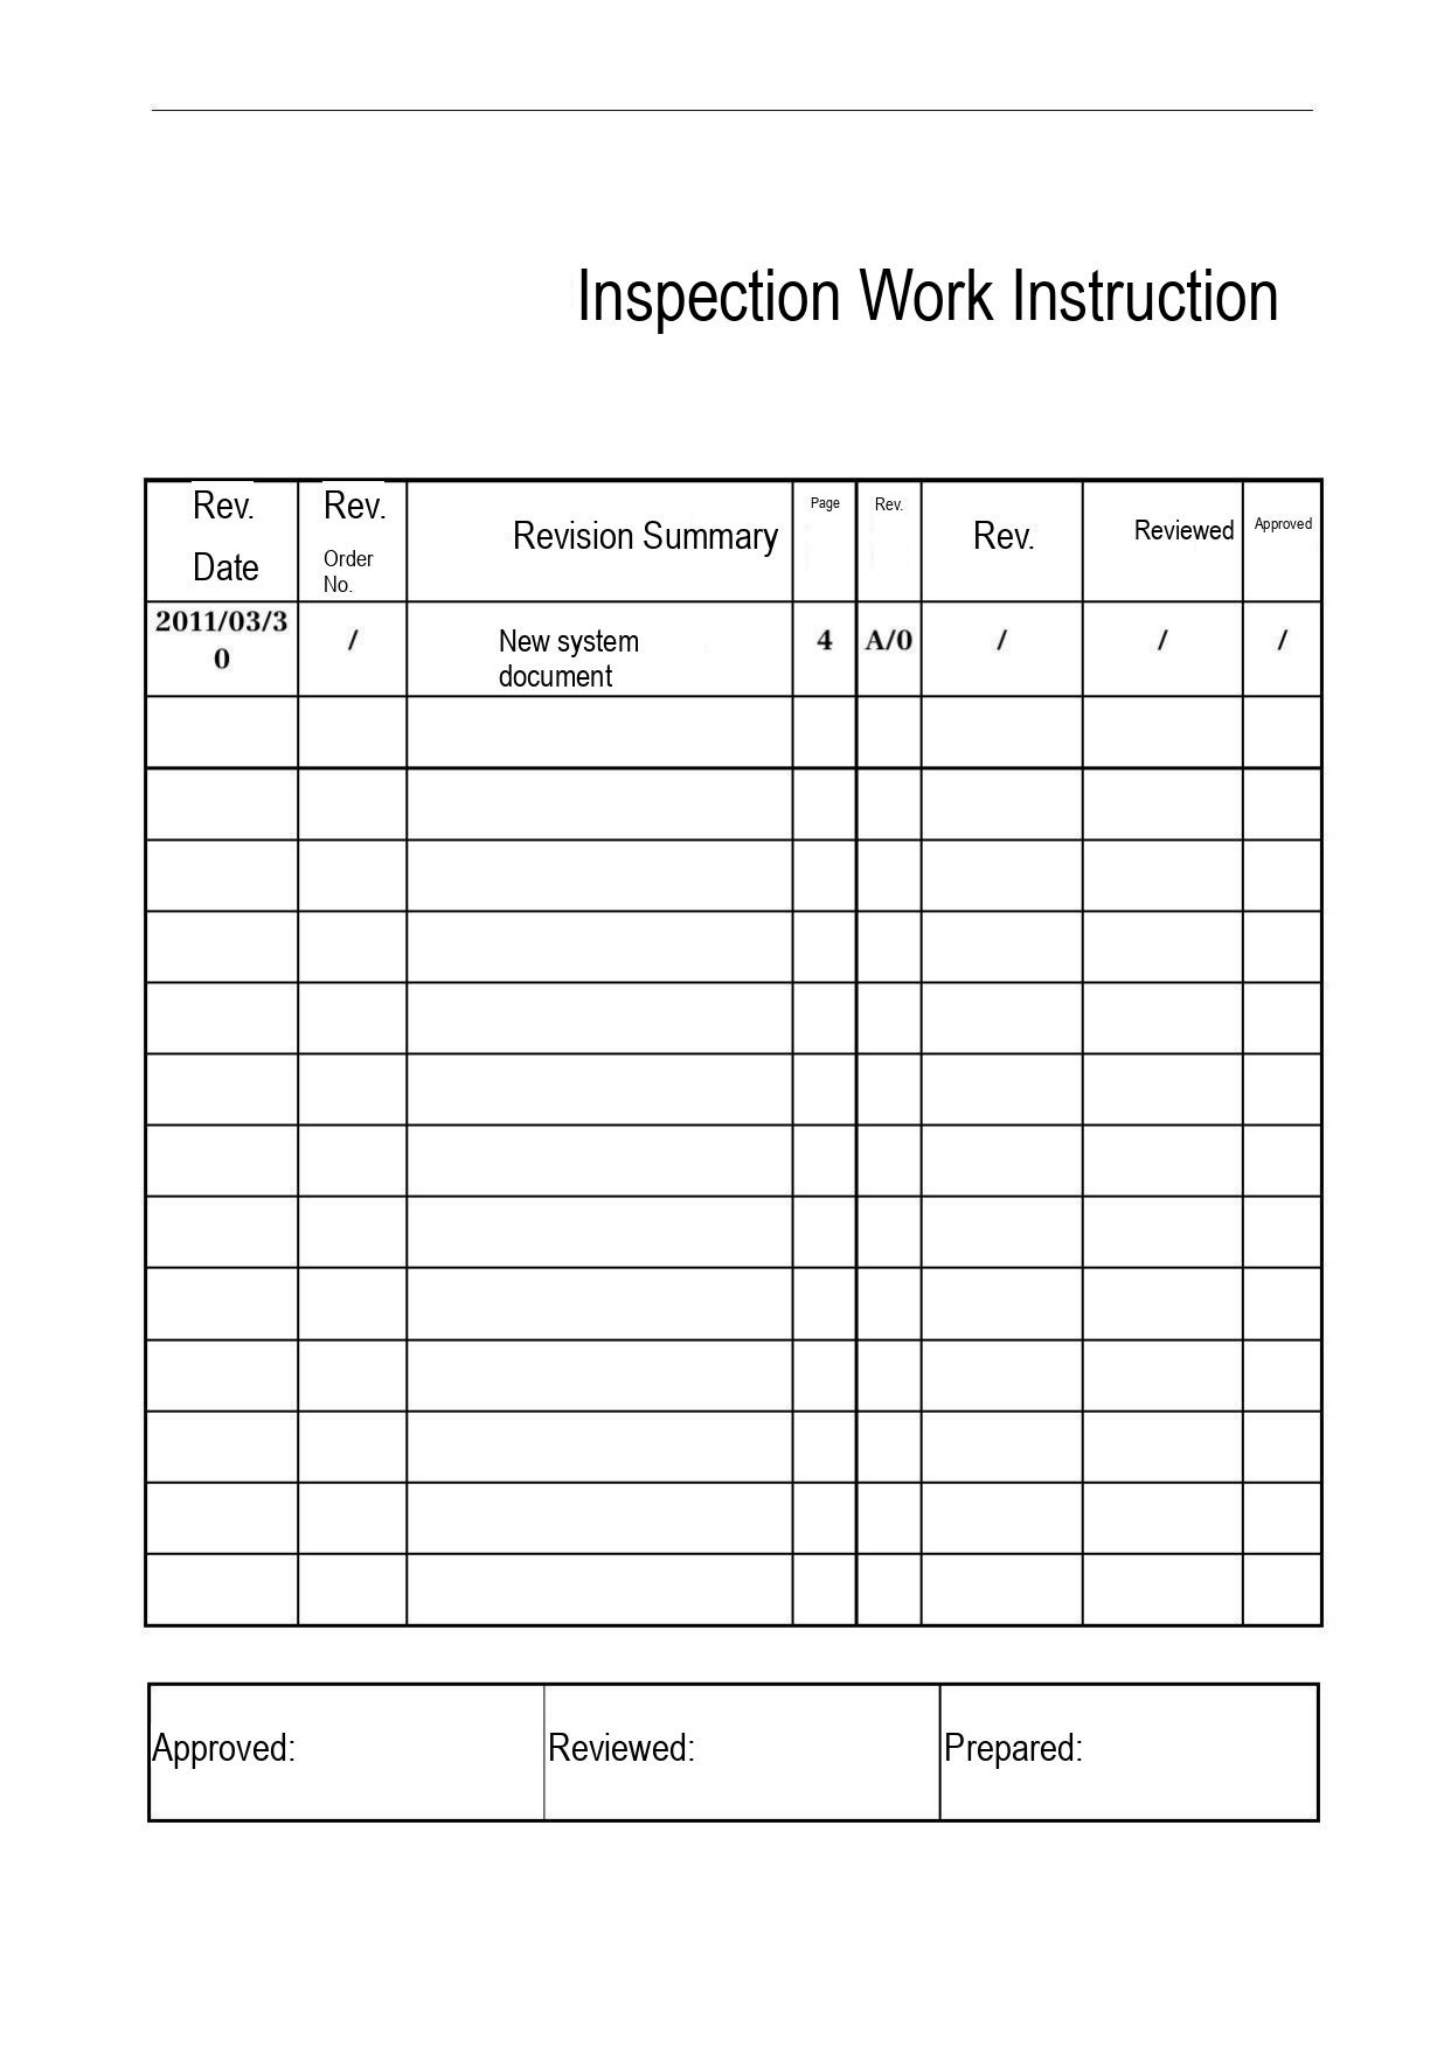Inspection Work Instruction

| Rev. Date | Rev. Order No. | Revision Summary | Page | Rev. | Rev. | Reviewed | Approved |
|---|---|---|---|---|---|---|---|
| 2011/03/30 | / | New system document | 4 | A/0 | / | / | / |
| | | | | | | | |
| | | | | | | | |
| | | | | | | | |
| | | | | | | | |
| | | | | | | | |
| | | | | | | | |
| | | | | | | | |
| | | | | | | | |
| | | | | | | | |
| | | | | | | | |
| | | | | | | | |
| | | | | | | | |
| | | | | | | | |

| Approved: | Reviewed: | Prepared: |
|---|---|---|
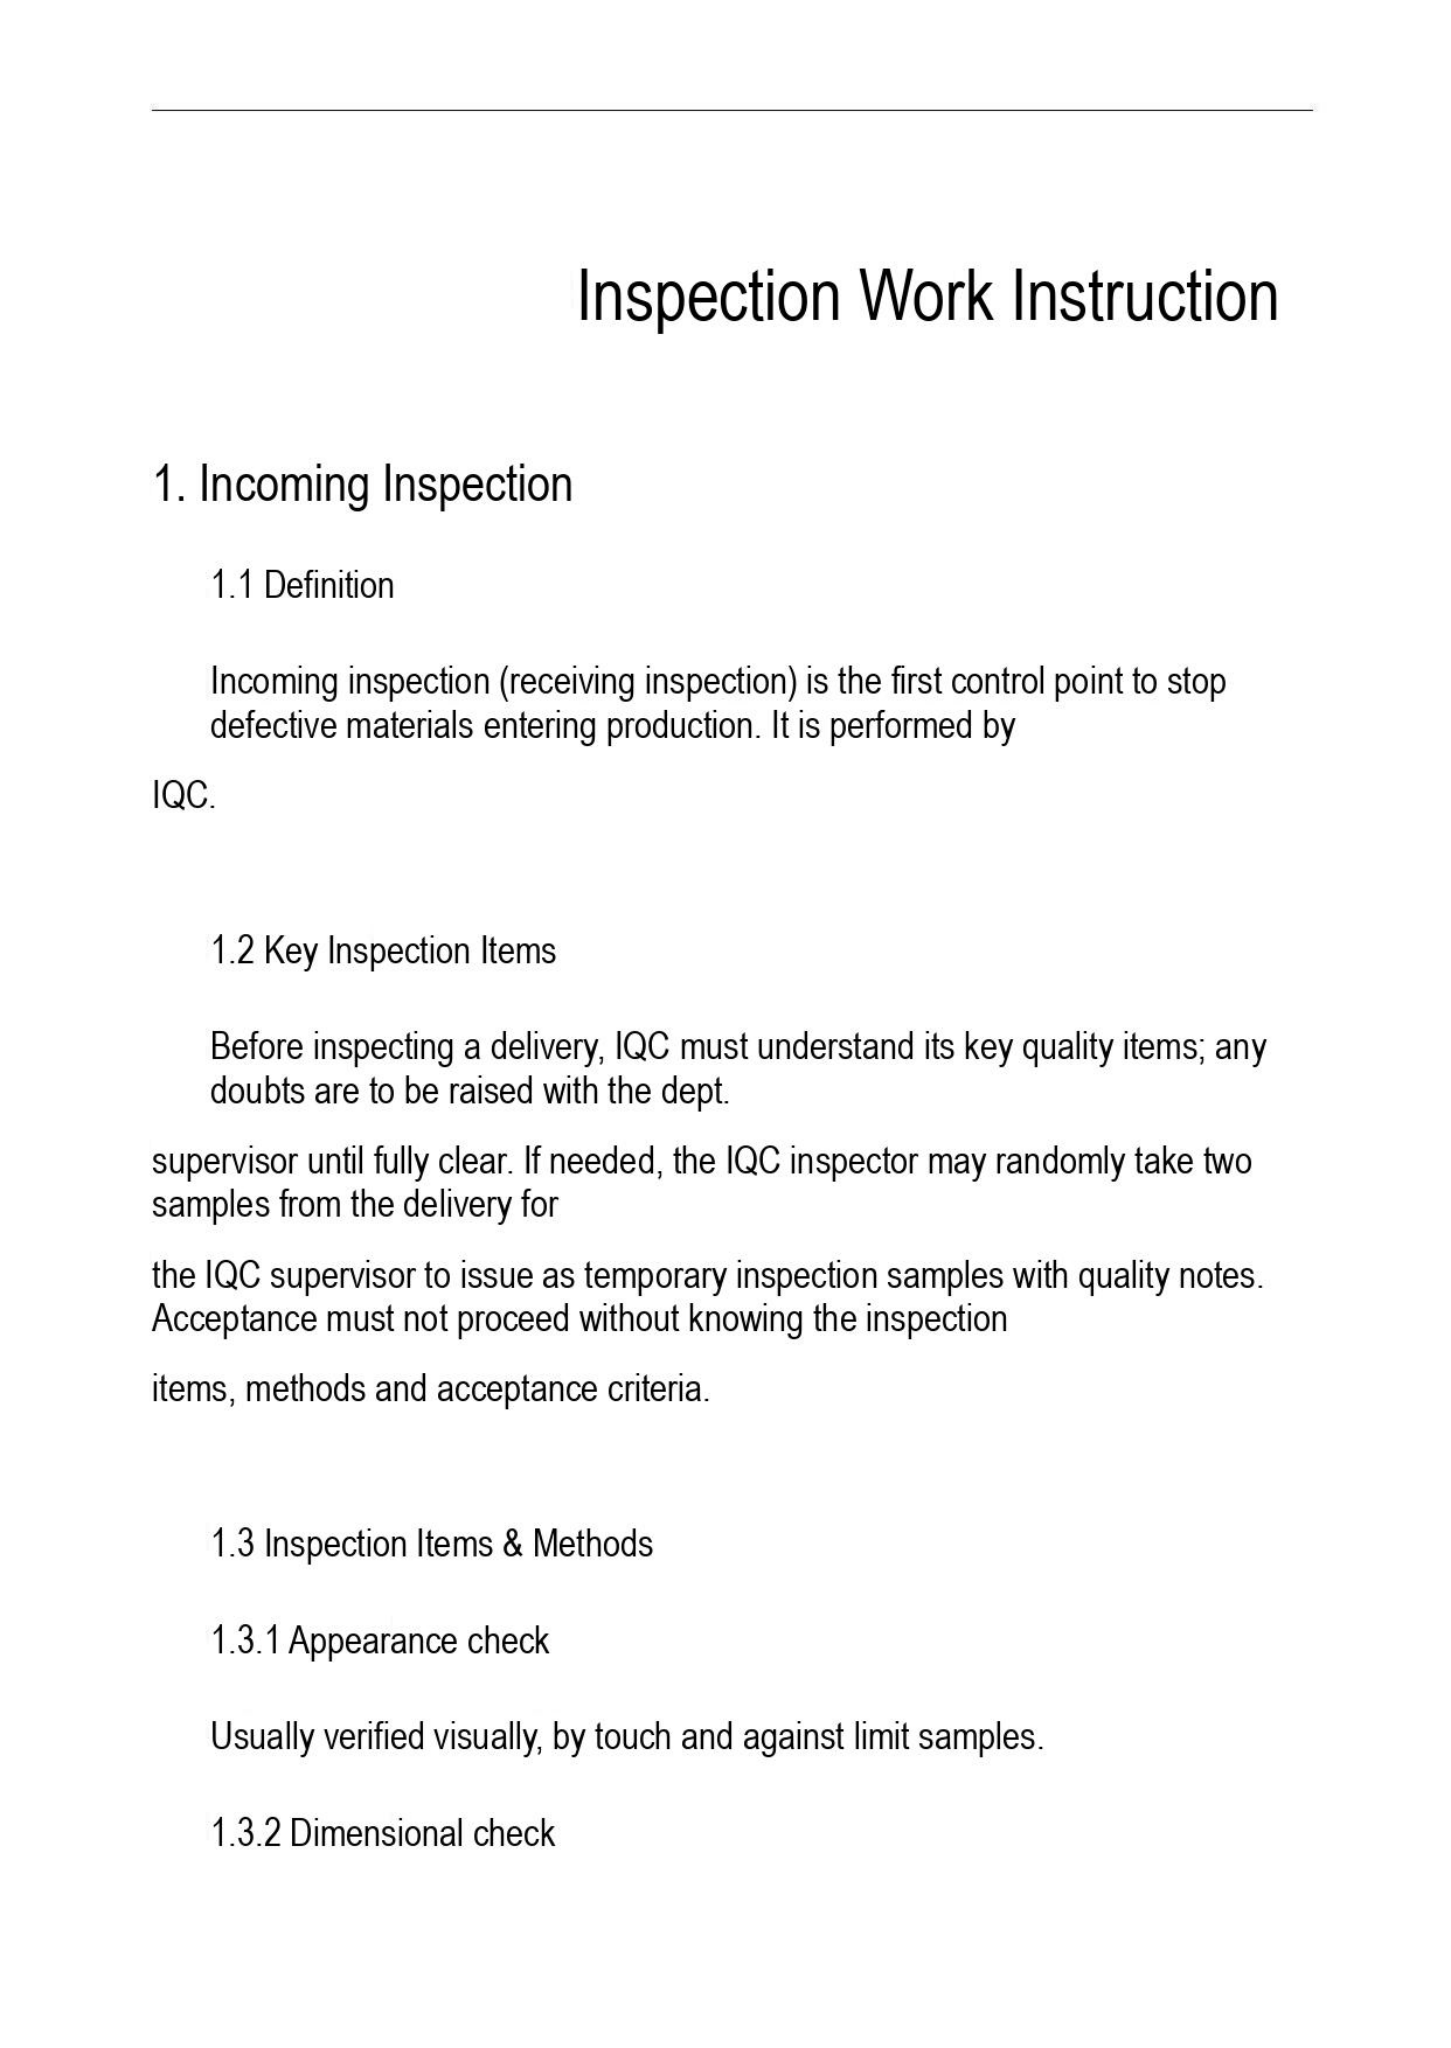Inspection Work Instruction

1. Incoming Inspection

1.1 Definition

Incoming inspection (receiving inspection) is the first control point to stop defective materials entering production. It is performed by IQC.

1.2 Key Inspection Items

Before inspecting a delivery, IQC must understand its key quality items; any doubts are to be raised with the dept. supervisor until fully clear. If needed, the IQC inspector may randomly take two samples from the delivery for the IQC supervisor to issue as temporary inspection samples with quality notes. Acceptance must not proceed without knowing the inspection items, methods and acceptance criteria.

1.3 Inspection Items & Methods

1.3.1 Appearance check

Usually verified visually, by touch and against limit samples.

1.3.2 Dimensional check
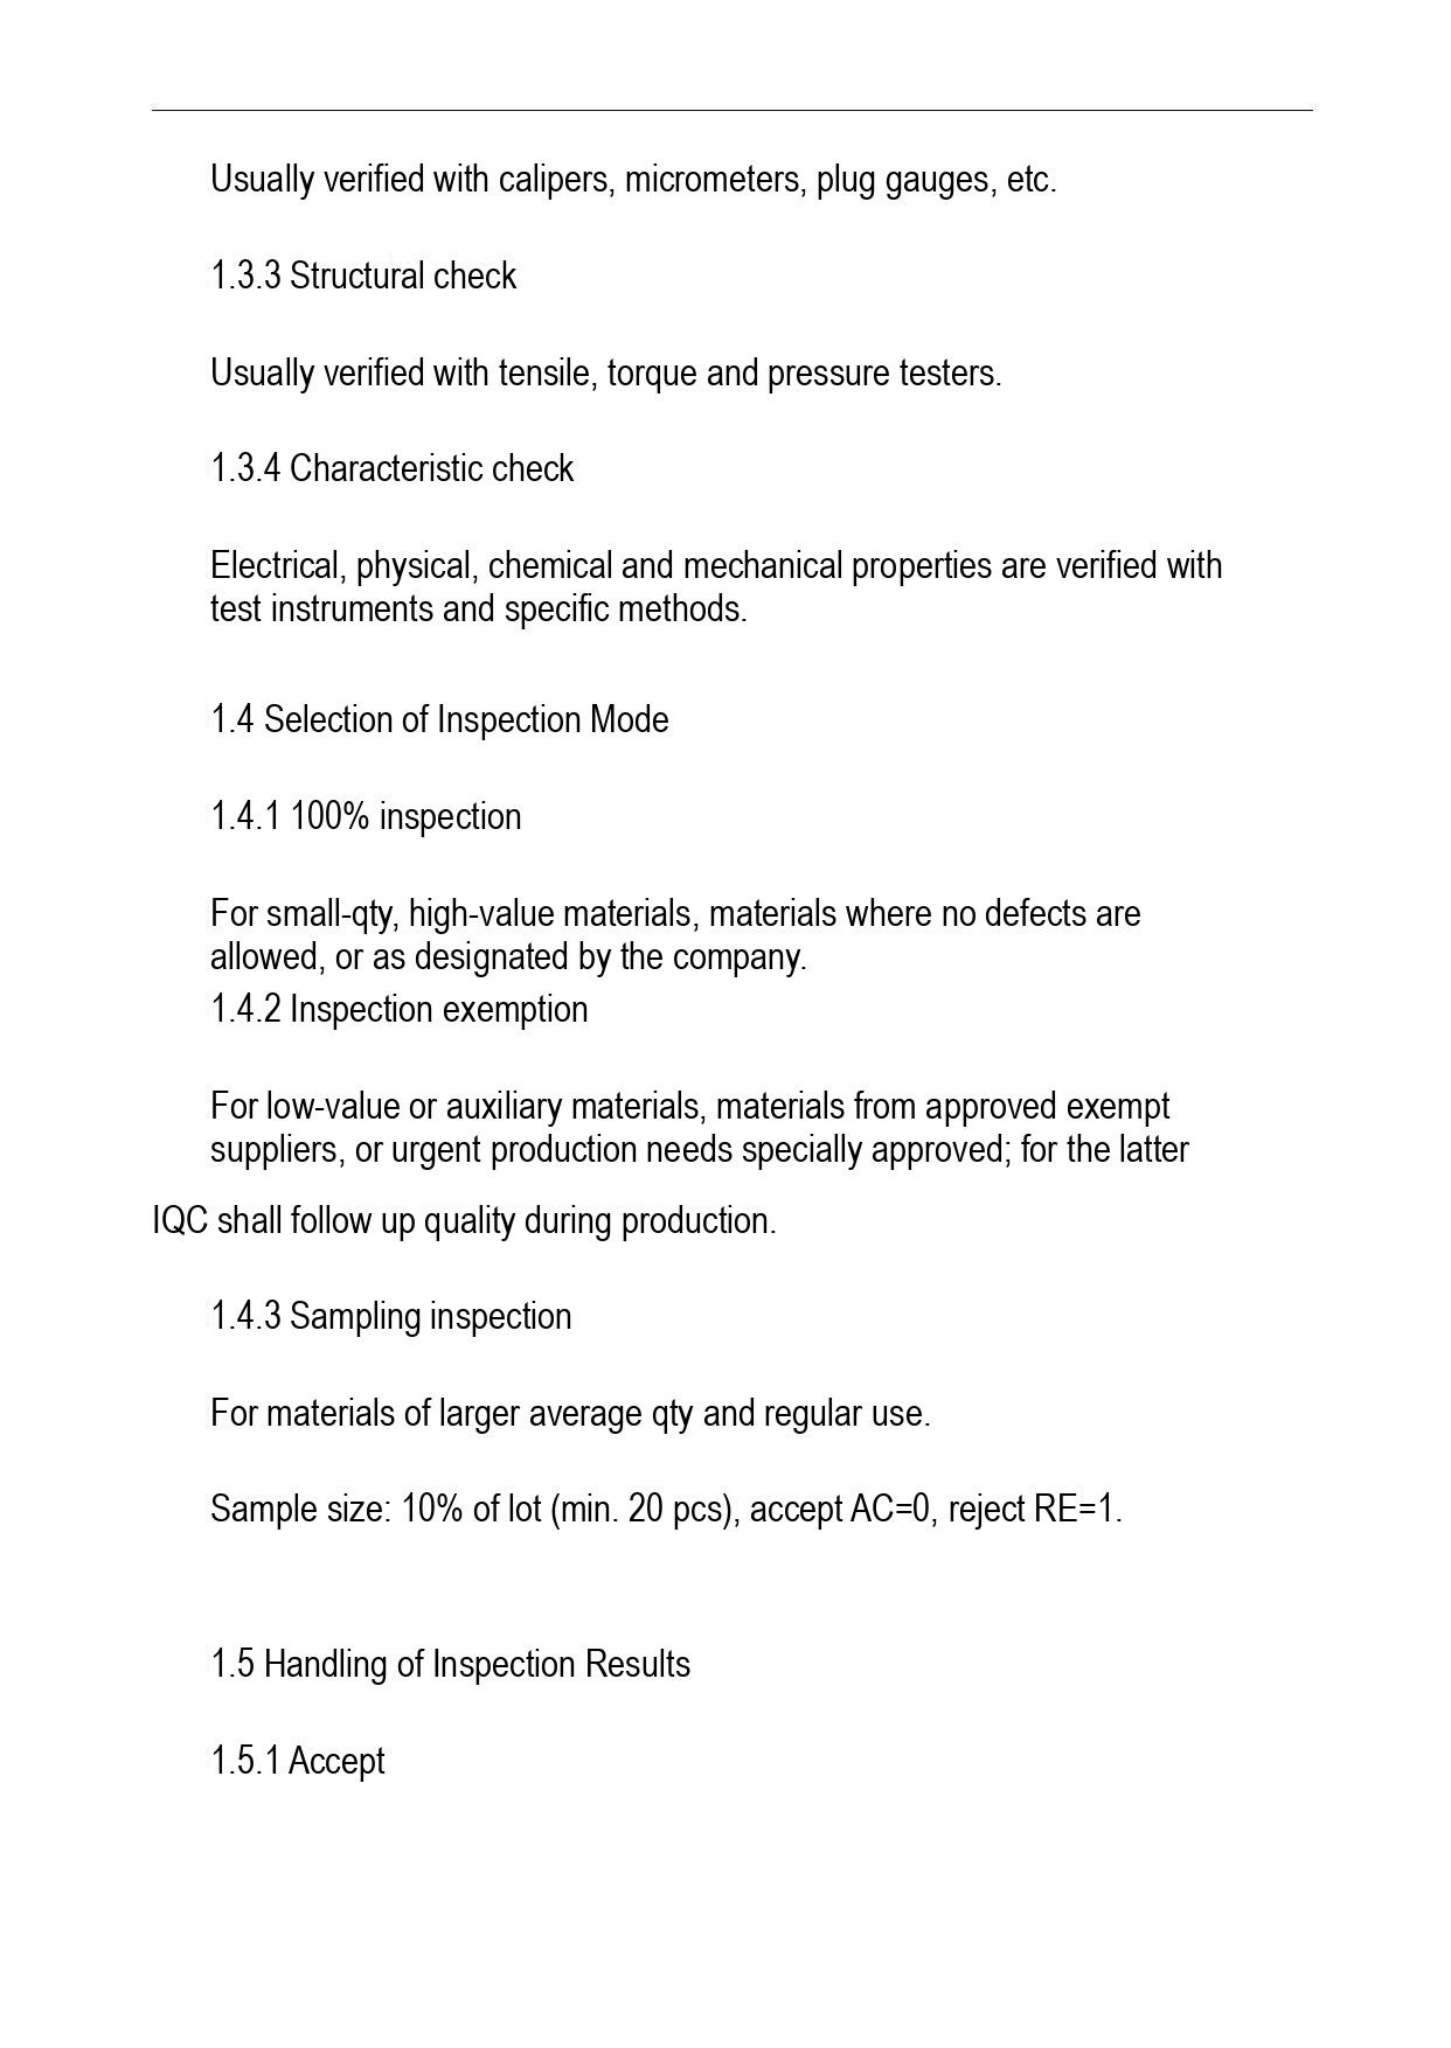Usually verified with calipers, micrometers, plug gauges, etc.

1.3.3 Structural check

Usually verified with tensile, torque and pressure testers.

1.3.4 Characteristic check

Electrical, physical, chemical and mechanical properties are verified with test instruments and specific methods.

1.4 Selection of Inspection Mode

1.4.1 100% inspection

For small-qty, high-value materials, materials where no defects are allowed, or as designated by the company.
1.4.2 Inspection exemption

For low-value or auxiliary materials, materials from approved exempt suppliers, or urgent production needs specially approved; for the latter

IQC shall follow up quality during production.

1.4.3 Sampling inspection

For materials of larger average qty and regular use.

Sample size: 10% of lot (min. 20 pcs), accept AC=0, reject RE=1.

1.5 Handling of Inspection Results

1.5.1 Accept
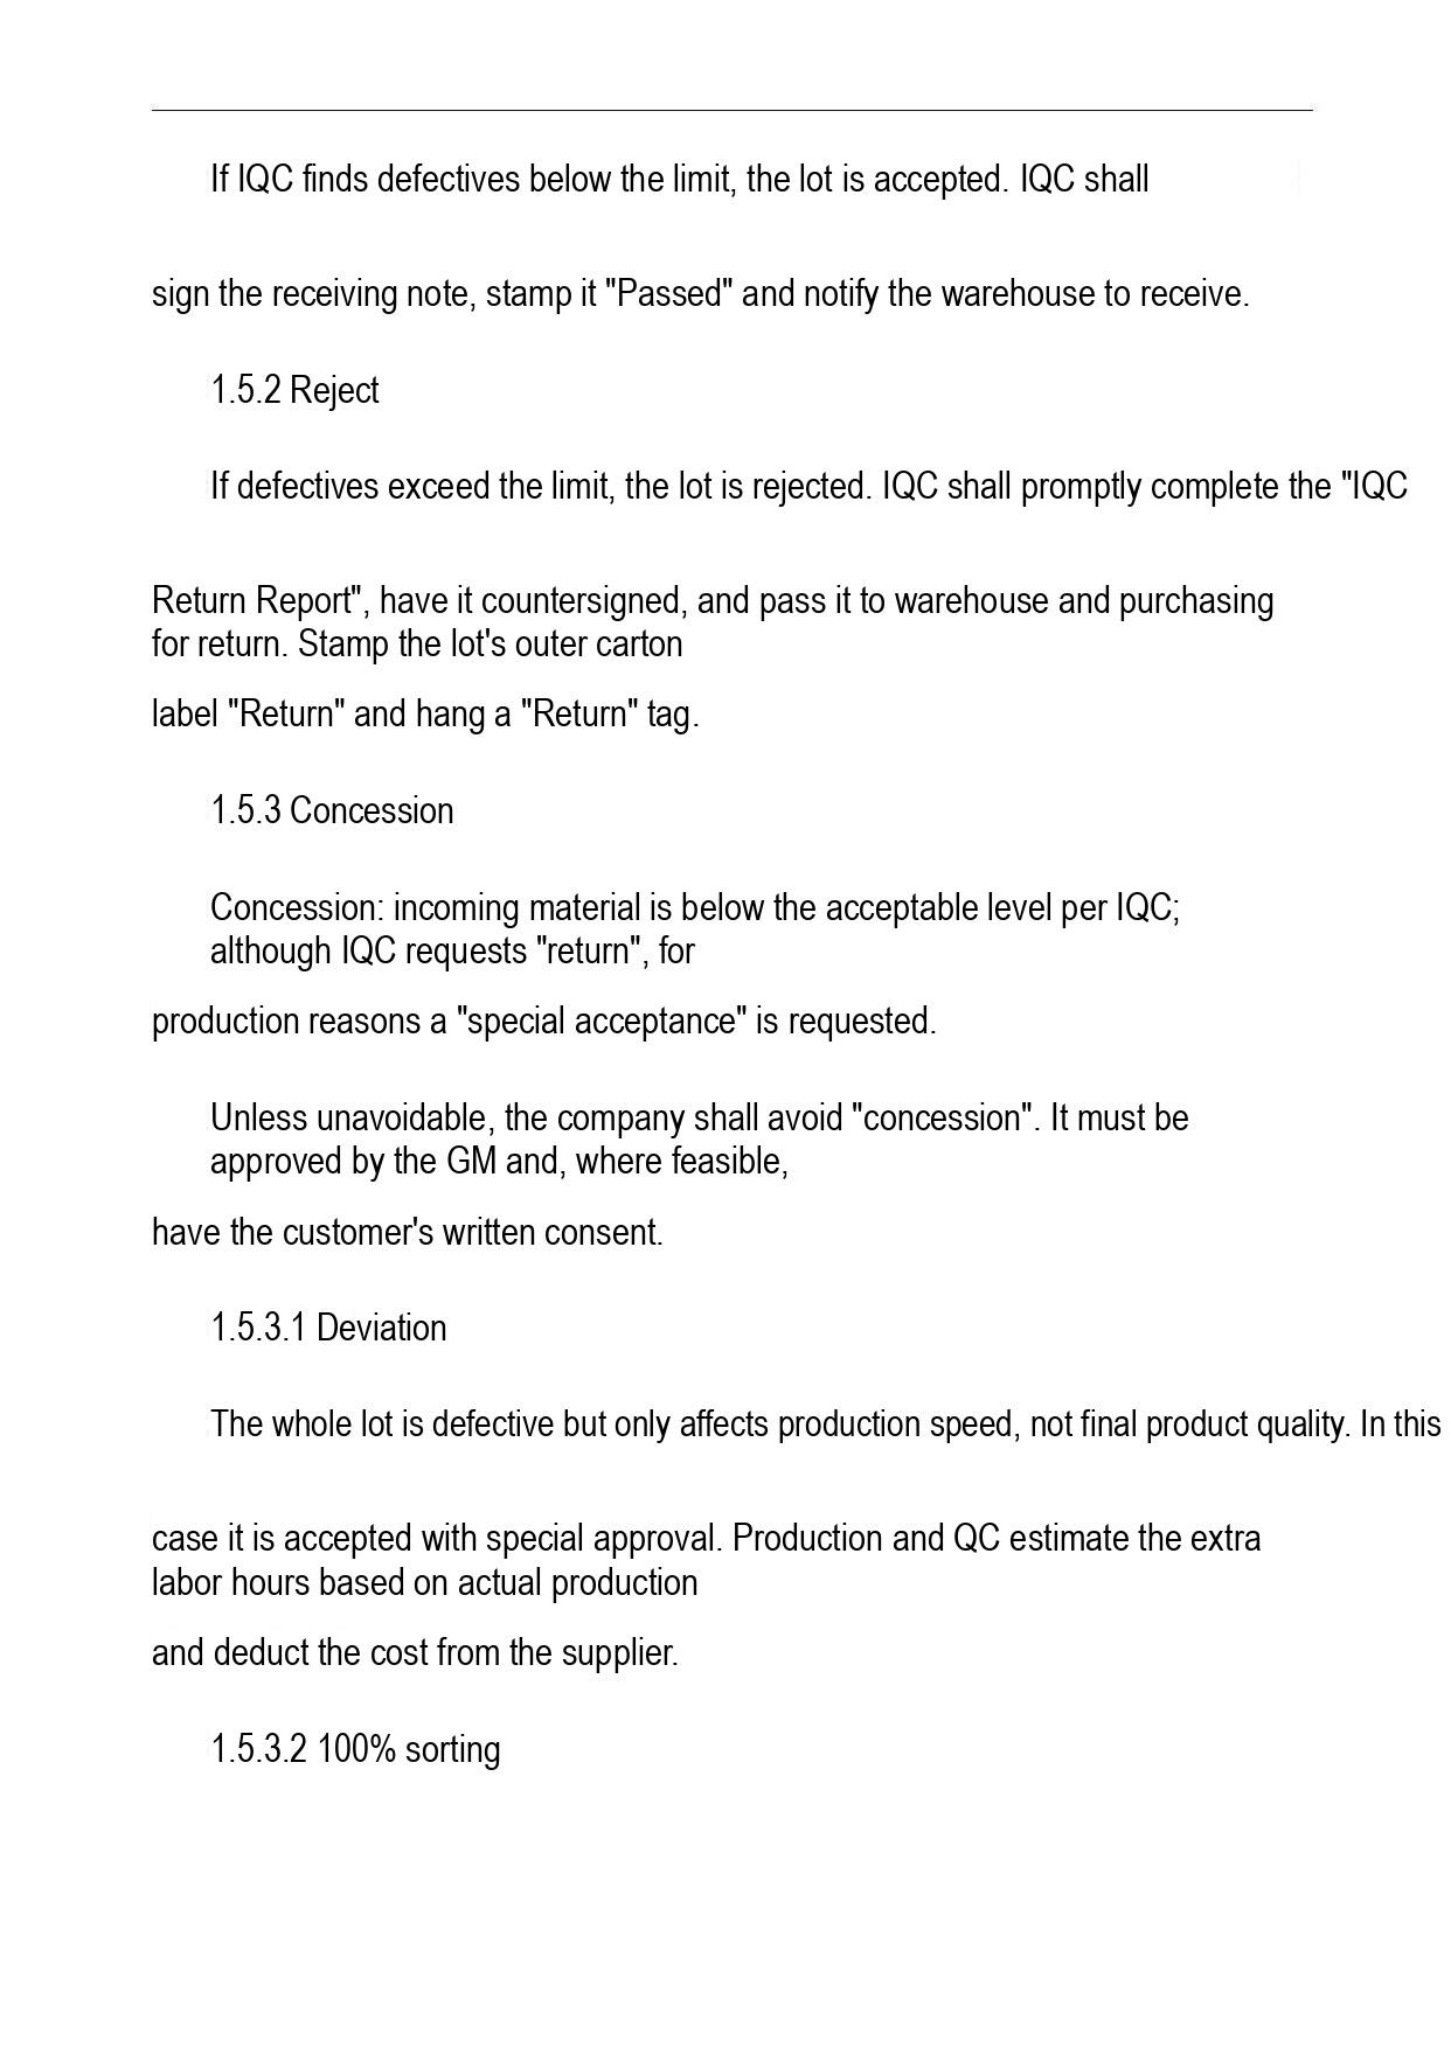If IQC finds defectives below the limit, the lot is accepted. IQC shall sign the receiving note, stamp it "Passed" and notify the warehouse to receive.

1.5.2 Reject

If defectives exceed the limit, the lot is rejected. IQC shall promptly complete the "IQC Return Report", have it countersigned, and pass it to warehouse and purchasing for return. Stamp the lot's outer carton label "Return" and hang a "Return" tag.

1.5.3 Concession

Concession: incoming material is below the acceptable level per IQC; although IQC requests "return", for production reasons a "special acceptance" is requested.

Unless unavoidable, the company shall avoid "concession". It must be approved by the GM and, where feasible, have the customer's written consent.

1.5.3.1 Deviation

The whole lot is defective but only affects production speed, not final product quality. In this case it is accepted with special approval. Production and QC estimate the extra labor hours based on actual production and deduct the cost from the supplier.

1.5.3.2 100% sorting
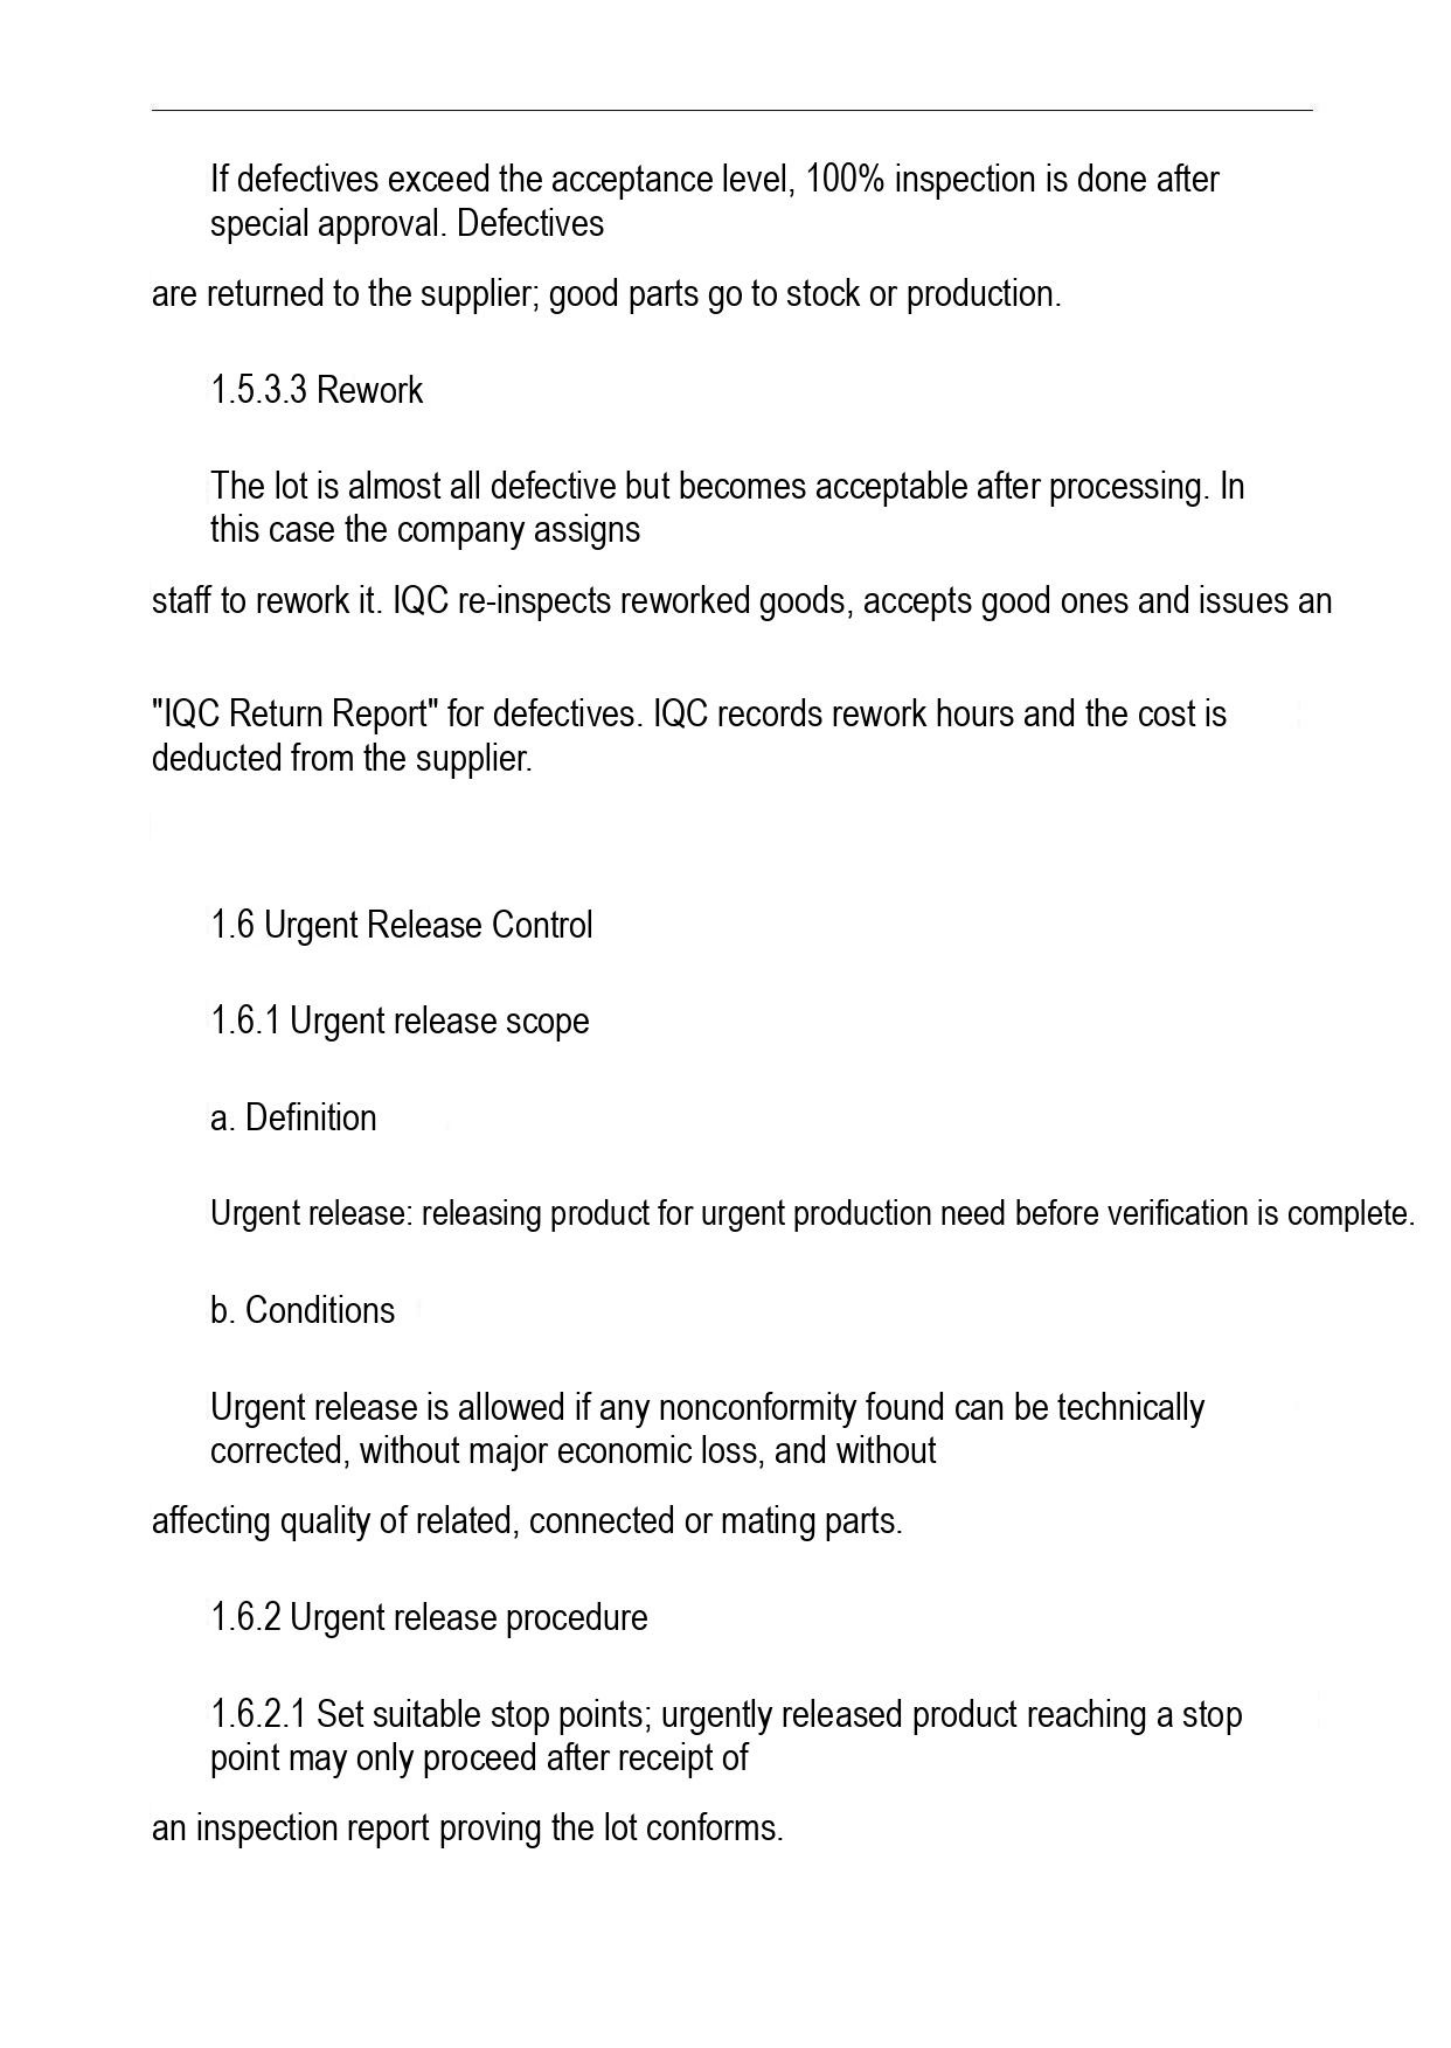If defectives exceed the acceptance level, 100% inspection is done after special approval. Defectives are returned to the supplier; good parts go to stock or production.

1.5.3.3 Rework

The lot is almost all defective but becomes acceptable after processing. In this case the company assigns staff to rework it. IQC re-inspects reworked goods, accepts good ones and issues an "IQC Return Report" for defectives. IQC records rework hours and the cost is deducted from the supplier.

1.6 Urgent Release Control

1.6.1 Urgent release scope

a. Definition

Urgent release: releasing product for urgent production need before verification is complete.

b. Conditions

Urgent release is allowed if any nonconformity found can be technically corrected, without major economic loss, and without affecting quality of related, connected or mating parts.

1.6.2 Urgent release procedure

1.6.2.1 Set suitable stop points; urgently released product reaching a stop point may only proceed after receipt of an inspection report proving the lot conforms.
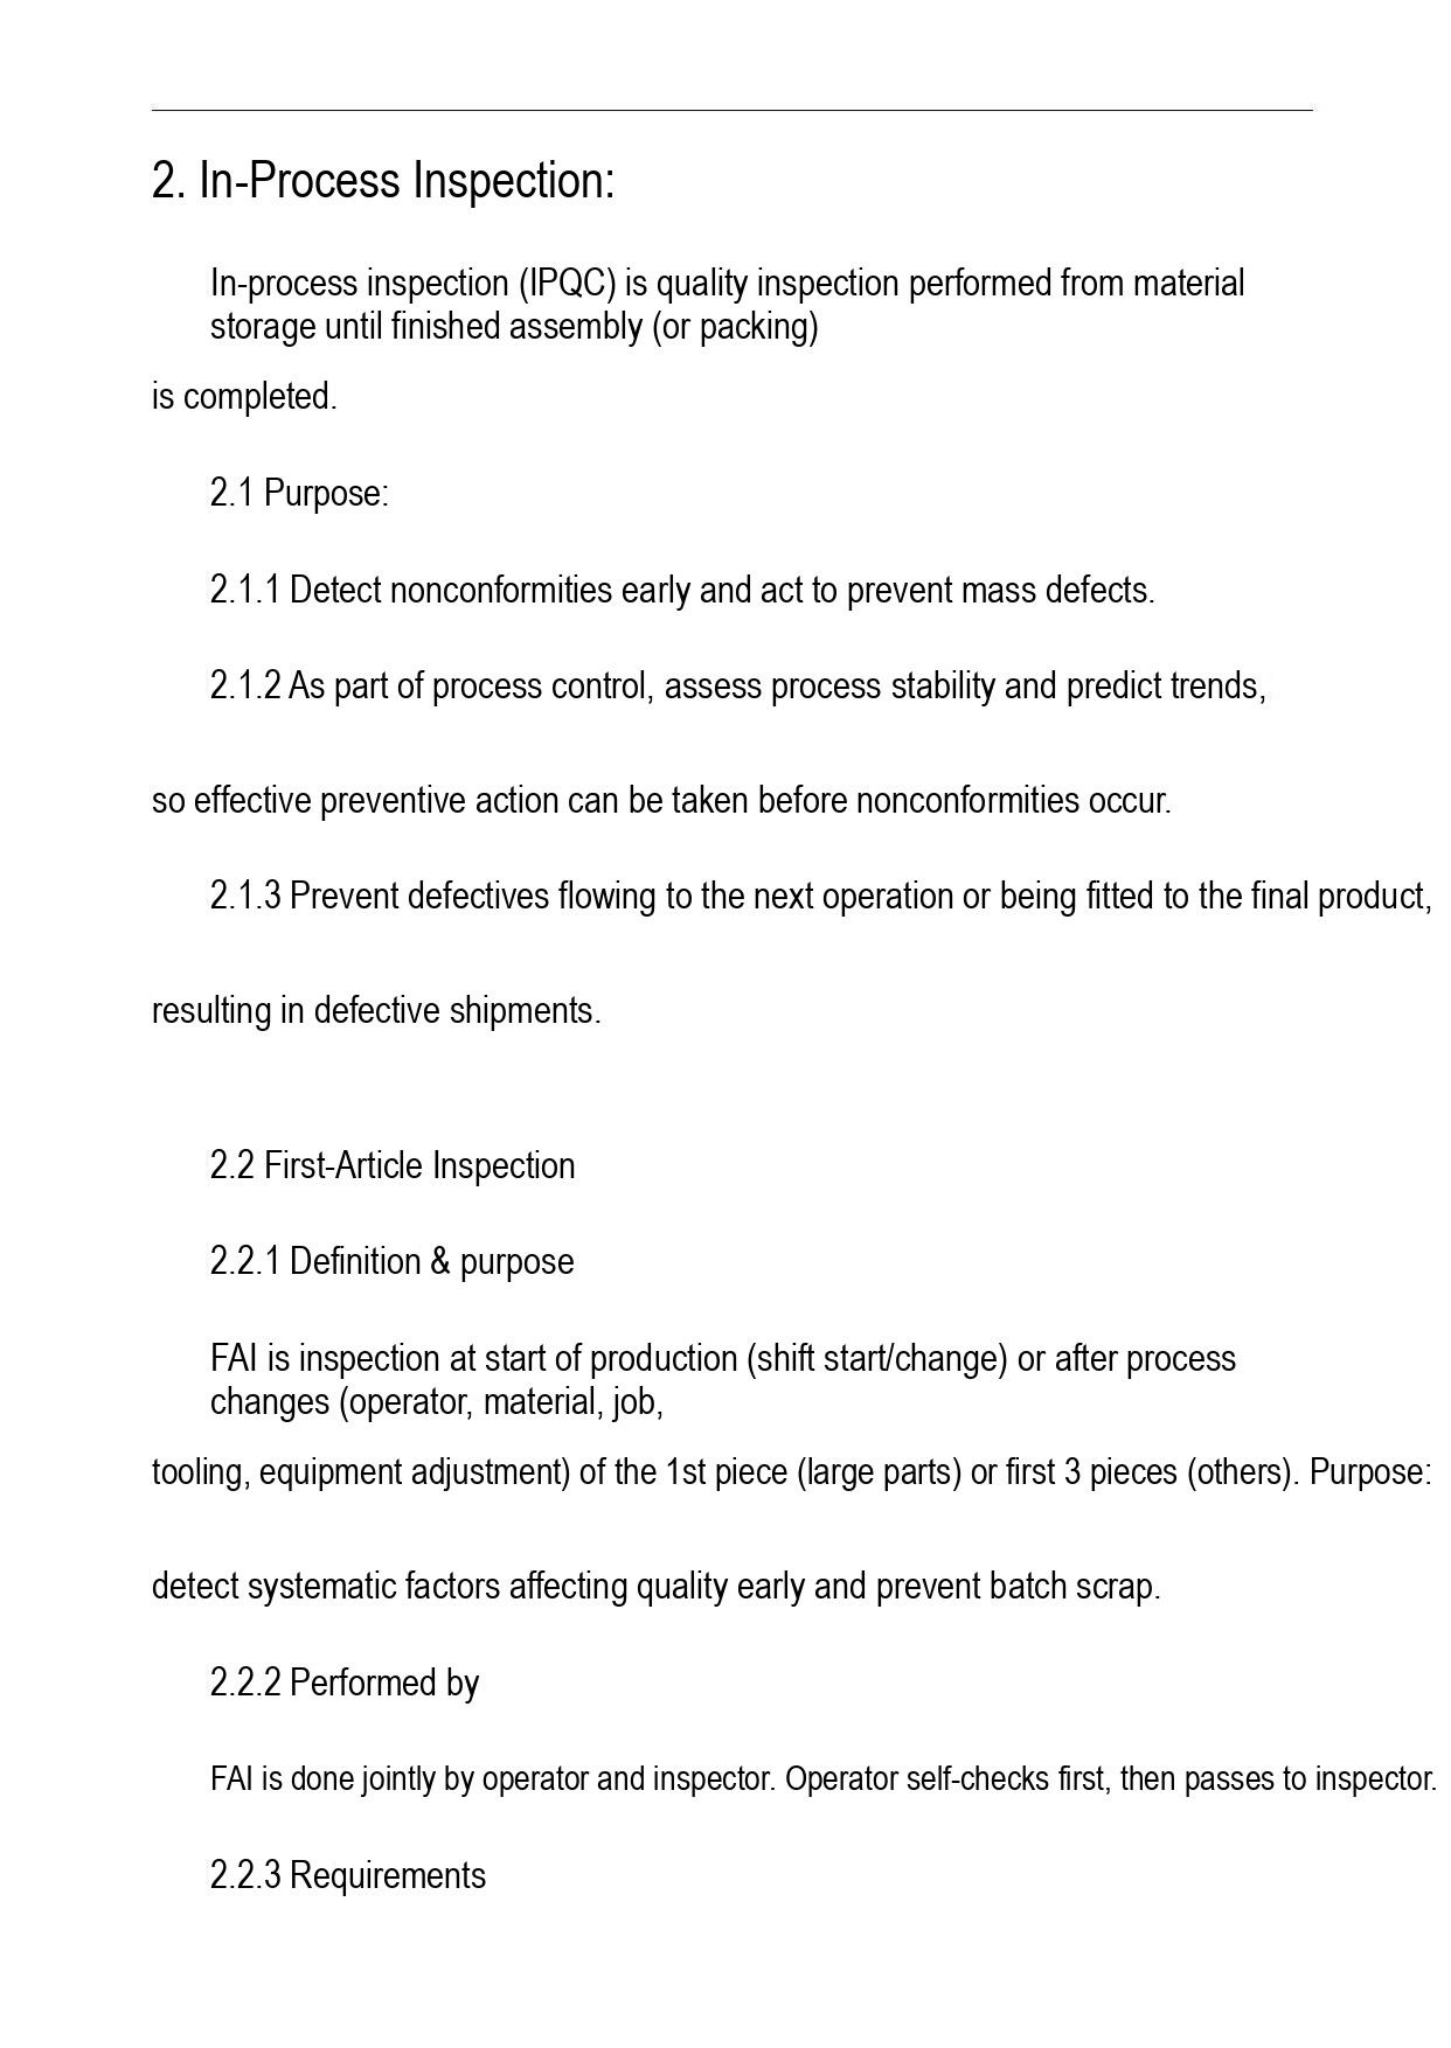# 2. In-Process Inspection:

In-process inspection (IPQC) is quality inspection performed from material storage until finished assembly (or packing) is completed.

2.1 Purpose:

2.1.1 Detect nonconformities early and act to prevent mass defects.

2.1.2 As part of process control, assess process stability and predict trends, so effective preventive action can be taken before nonconformities occur.

2.1.3 Prevent defectives flowing to the next operation or being fitted to the final product, resulting in defective shipments.

2.2 First-Article Inspection

2.2.1 Definition & purpose

FAI is inspection at start of production (shift start/change) or after process changes (operator, material, job, tooling, equipment adjustment) of the 1st piece (large parts) or first 3 pieces (others). Purpose: detect systematic factors affecting quality early and prevent batch scrap.

2.2.2 Performed by

FAI is done jointly by operator and inspector. Operator self-checks first, then passes to inspector.

2.2.3 Requirements
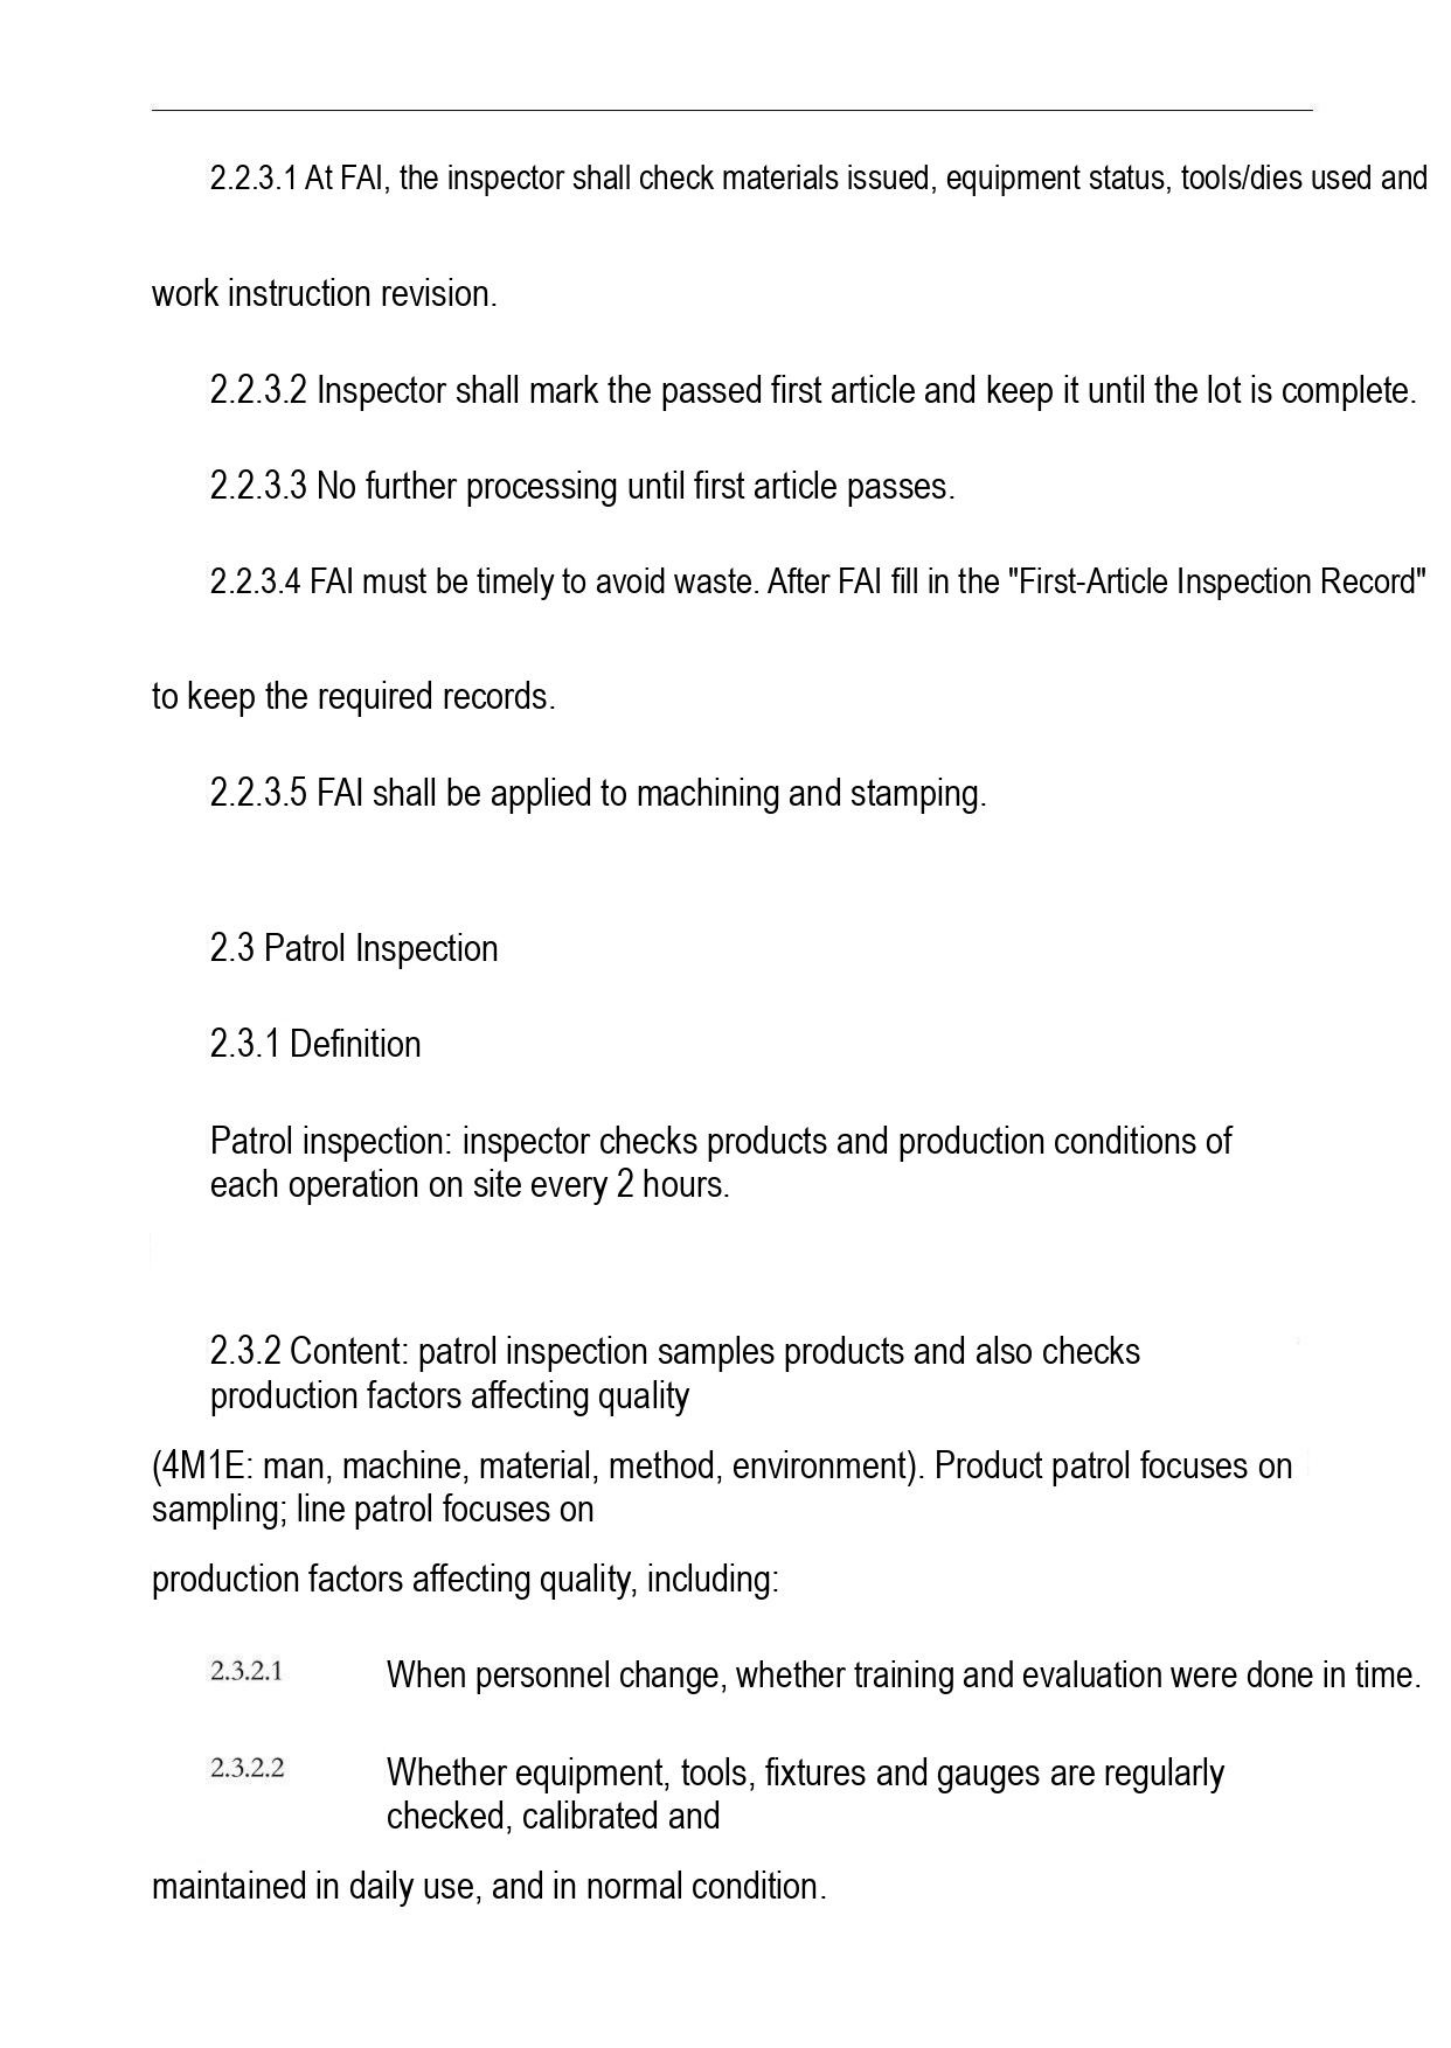2.2.3.1 At FAI, the inspector shall check materials issued, equipment status, tools/dies used and work instruction revision.

2.2.3.2 Inspector shall mark the passed first article and keep it until the lot is complete.

2.2.3.3 No further processing until first article passes.

2.2.3.4 FAI must be timely to avoid waste. After FAI fill in the "First-Article Inspection Record" to keep the required records.

2.2.3.5 FAI shall be applied to machining and stamping.

2.3 Patrol Inspection

2.3.1 Definition

Patrol inspection: inspector checks products and production conditions of each operation on site every 2 hours.

2.3.2 Content: patrol inspection samples products and also checks production factors affecting quality (4M1E: man, machine, material, method, environment). Product patrol focuses on sampling; line patrol focuses on production factors affecting quality, including:

2.3.2.1 When personnel change, whether training and evaluation were done in time.

2.3.2.2 Whether equipment, tools, fixtures and gauges are regularly checked, calibrated and maintained in daily use, and in normal condition.